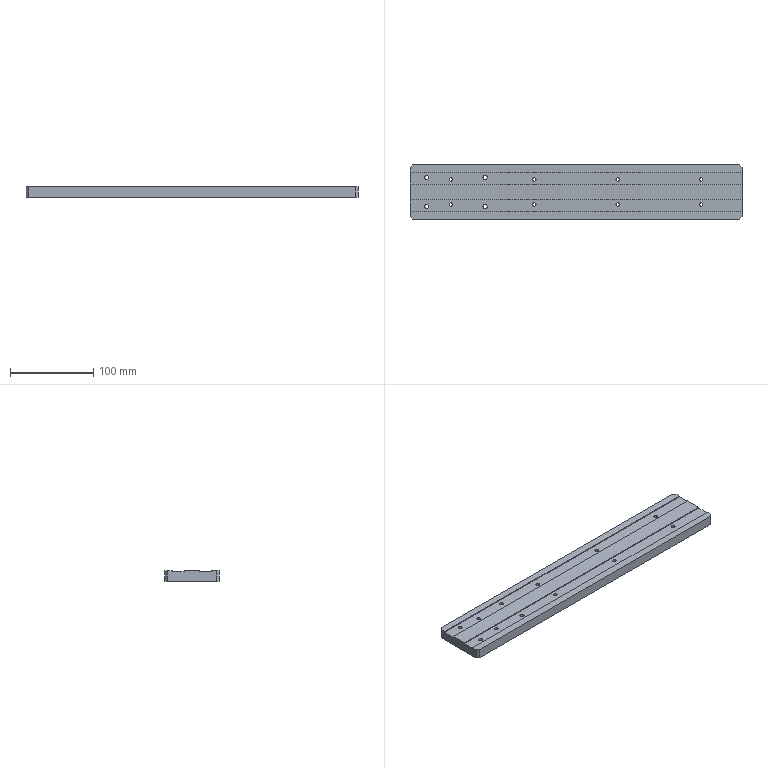Part | STEP file | PN_0017 | 1 solid | 42 faces | box 398 x 65 x 12 mm | volume 296877 mm3 | cylinder 24 | plane 18 | commonest cylinder face diameters 4.2 x16 5 x8